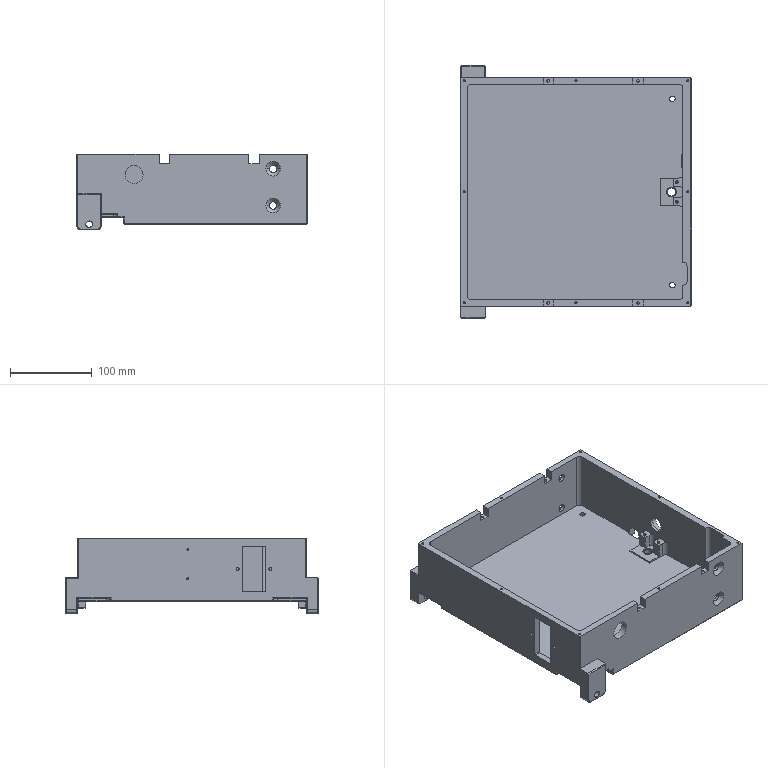NC program | Mastercam | posted with a generic post
Lines 7234 to 8037 of 104433:
(20 FEM |TOOL - 20|DIA. OFF. - 20|LEN. - 20|TOOL DIA. - 20.)
N4630 T20 M6
N4632 G0 G54 G90 X-117.9 Y-104.336 C0. B0. S4000 M3
N4634 G43 H20 Z50.
N4636 Z2.61
N4638 G1 Z2.11 F600.
N4640 X-117.911 Z1.901 F4000.
N4642 X-117.944 Z1.694
N4644 X-117.998 Z1.492
N4646 X-118.073 Z1.296
N4648 X-118.168 Z1.11
N4650 X-118.282 Z.934
N4652 X-118.414 Z.771
N4654 X-118.562 Z.623
N4656 X-118.724 Z.492
N4658 X-118.9 Z.378
N4660 X-119.087 Z.283
N4662 X-119.282 Z.208
N4664 X-119.484 Z.153
N4666 X-119.691 Z.121
N4668 X-119.9 Z.11
N4670 X-120.109 Y-104.347 Z.102
N4672 X-120.316 Y-104.38 Z.095
N4674 X-120.518 Y-104.434 Z.088
N4676 X-120.713 Y-104.509 Z.08
N4678 X-120.9 Y-104.604 Z.073
N4680 X-121.076 Y-104.718 Z.066
N4682 X-121.238 Y-104.85 Z.059
N4684 X-121.386 Y-104.998 Z.051
N4686 X-121.518 Y-105.161 Z.044
N4688 X-121.632 Y-105.336 Z.037
N4690 X-121.727 Y-105.523 Z.029
N4692 X-121.802 Y-105.718 Z.022
N4694 X-121.856 Y-105.92 Z.015
N4696 X-121.889 Y-106.127 Z.007
N4698 X-121.9 Y-106.336 Z0.
N4700 Y-120.9
N4702 G2 X-120.453 Y-120.899 I1.447 J-1517.237
N4704 X-113.75 Y-120.914 J-1517.238
N4706 X-110.741 Y-121.53 I-.477 J-9.989
N4708 G1 X-110.718 Y-121.538
N4710 G2 X-108.631 Y-122.608 I-3.486 J-9.373
N4712 G1 X-108.612 Y-122.621
N4714 G2 X-106.882 Y-124.093 I-5.573 J-8.303
N4716 G1 X-106.866 Y-124.109
N4718 G2 X-105.533 Y-125.9 I-7.304 J-6.831
N4720 G1 X-94.468
N4722 X-94.196 Y-125.462
N4724 G2 X-93.088 Y-124.06 I8.366 J-5.478
N4726 G1 X-93.072 Y-124.044
N4728 G2 X-91.448 Y-122.661 I7.258 J-6.879
N4730 G1 X-91.431 Y-122.65
N4732 G2 X-89.722 Y-121.714 I5.633 J-8.262
N4734 G1 X-89.705 Y-121.707
N4736 G2 X-87.923 Y-121.137 I3.925 J-9.198
N4738 G1 X-87.904 Y-121.133
N4740 G2 X-85.963 Y-120.903 I2.142 J-9.768
N4742 G1 X-85.271 Y-120.9
N4744 X-85.062 Y-120.888 Z.007
N4746 X-84.855 Y-120.855 Z.015
N4748 X-84.653 Y-120.8 Z.022
N4750 X-84.458 Y-120.724 Z.029
N4752 X-84.272 Y-120.628 Z.037
N4754 X-84.097 Y-120.513 Z.044
N4756 X-83.935 Y-120.381 Z.051
N4758 X-83.787 Y-120.232 Z.059
N4760 X-83.656 Y-120.069 Z.066
N4762 X-83.543 Y-119.893 Z.073
N4764 X-83.449 Y-119.706 Z.08
N4766 X-83.374 Y-119.51 Z.088
N4768 X-83.321 Y-119.308 Z.095
N4770 X-83.289 Y-119.101 Z.102
N4772 X-83.279 Y-118.892 Z.11
N4774 X-83.28 Y-118.683 Z.121
N4776 X-83.281 Y-118.476 Z.153
N4778 Y-118.274 Z.208
N4780 X-83.282 Y-118.079 Z.283
N4782 X-83.283 Y-117.892 Z.378
N4784 X-83.284 Y-117.716 Z.492
N4786 Y-117.554 Z.623
N4788 X-83.285 Y-117.406 Z.771
N4790 X-83.286 Y-117.274 Z.934
N4792 Y-117.16 Z1.11
N4794 Y-117.065 Z1.296
N4796 X-83.287 Y-116.99 Z1.492
N4798 Y-116.936 Z1.694
N4800 Y-116.903 Z1.901
N4802 Y-116.892 Z2.11
N4804 Z2.61
N4806 Z2.86
N4808 Z1.61
N4810 Z1.11 F600.
N4812 Y-116.903 Z.901 F4000.
N4814 Y-116.936 Z.694
N4816 Y-116.99 Z.492
N4818 X-83.286 Y-117.065 Z.296
N4820 Y-117.16 Z.11
N4822 Y-117.274 Z-.066
N4824 X-83.285 Y-117.406 Z-.229
N4826 X-83.284 Y-117.554 Z-.377
N4828 Y-117.716 Z-.508
N4830 X-83.283 Y-117.892 Z-.622
N4832 X-83.282 Y-118.079 Z-.717
N4834 X-83.281 Y-118.274 Z-.792
N4836 Y-118.476 Z-.847
N4838 X-83.28 Y-118.683 Z-.879
N4840 X-83.279 Y-118.892 Z-.89
N4842 X-83.289 Y-119.101 Z-.898
N4844 X-83.321 Y-119.308 Z-.905
N4846 X-83.374 Y-119.51 Z-.912
N4848 X-83.449 Y-119.706 Z-.92
N4850 X-83.543 Y-119.893 Z-.927
N4852 X-83.656 Y-120.069 Z-.934
N4854 X-83.787 Y-120.232 Z-.941
N4856 X-83.935 Y-120.381 Z-.949
N4858 X-84.097 Y-120.513 Z-.956
N4860 X-84.272 Y-120.628 Z-.963
N4862 X-84.458 Y-120.724 Z-.971
N4864 X-84.653 Y-120.8 Z-.978
N4866 X-84.855 Y-120.855 Z-.985
N4868 X-85.062 Y-120.888 Z-.993
N4870 X-85.271 Y-120.9 Z-1.
N4872 X-85.963 Y-120.903
N4874 G3 X-87.904 Y-121.133 I.201 J-9.998
N4876 G1 X-87.923 Y-121.137
N4878 G3 X-89.705 Y-121.707 I2.143 J-9.768
N4880 G1 X-89.722 Y-121.714
N4882 G3 X-91.431 Y-122.65 I3.924 J-9.198
N4884 G1 X-91.448 Y-122.661
N4886 G3 X-93.072 Y-124.044 I5.634 J-8.262
N4888 G1 X-93.088 Y-124.06
N4890 G3 X-94.196 Y-125.462 I7.258 J-6.88
N4892 G1 X-94.468 Y-125.9
N4894 X-105.533
N4896 G3 X-106.866 Y-124.109 I-8.637 J-5.04
N4898 G1 X-106.882 Y-124.093
N4900 G3 X-108.612 Y-122.621 I-7.303 J-6.831
N4902 G1 X-108.631 Y-122.608
N4904 G3 X-110.718 Y-121.538 I-5.573 J-8.303
N4906 G1 X-110.741 Y-121.53
N4908 G3 X-113.75 Y-120.914 I-3.486 J-9.373
N4910 X-120.453 Y-120.899 I-6.703 J-1517.224
N4912 X-121.9 Y-120.9 J-1517.239
N4914 G1 Y-106.336
N4916 X-121.875 Y-106.023 Z-.989
N4918 X-121.802 Y-105.718 Z-.978
N4920 X-121.682 Y-105.428 Z-.967
N4922 X-121.518 Y-105.161 Z-.956
N4924 X-121.314 Y-104.922 Z-.945
N4926 X-121.076 Y-104.718 Z-.934
N4928 X-120.808 Y-104.554 Z-.923
N4930 X-120.518 Y-104.434 Z-.912
N4932 X-120.213 Y-104.361 Z-.901
N4934 X-119.9 Y-104.336 Z-.89
N4936 X-119.691 Z-.879
N4938 X-119.484 Z-.847
N4940 X-119.282 Z-.792
N4942 X-119.087 Z-.717
N4944 X-118.9 Z-.622
N4946 X-118.724 Z-.508
N4948 X-118.562 Z-.377
N4950 X-118.414 Z-.229
N4952 X-118.282 Z-.066
N4954 X-118.168 Z.11
N4956 X-118.073 Z.296
N4958 X-117.998 Z.492
N4960 X-117.944 Z.694
N4962 X-117.911 Z.901
N4964 X-117.9 Z1.11
N4966 Z1.61
N4968 Z1.86
N4970 Z.61
N4972 Z.11 F600.
N4974 X-117.911 Z-.099 F4000.
N4976 X-117.944 Z-.306
N4978 X-117.998 Z-.508
N4980 X-118.073 Z-.704
N4982 X-118.168 Z-.89
N4984 X-118.282 Z-1.066
N4986 X-118.414 Z-1.229
N4988 X-118.562 Z-1.377
N4990 X-118.724 Z-1.508
N4992 X-118.9 Z-1.622
N4994 X-119.087 Z-1.717
N4996 X-119.282 Z-1.792
N4998 X-119.484 Z-1.847
N5000 X-119.691 Z-1.879
N5002 X-119.9 Z-1.89
N5004 X-120.109 Y-104.347 Z-1.898
N5006 X-120.316 Y-104.38 Z-1.905
N5008 X-120.518 Y-104.434 Z-1.912
N5010 X-120.713 Y-104.509 Z-1.92
N5012 X-120.9 Y-104.604 Z-1.927
N5014 X-121.076 Y-104.718 Z-1.934
N5016 X-121.238 Y-104.85 Z-1.941
N5018 X-121.386 Y-104.998 Z-1.949
N5020 X-121.518 Y-105.161 Z-1.956
N5022 X-121.632 Y-105.336 Z-1.963
N5024 X-121.727 Y-105.523 Z-1.971
N5026 X-121.802 Y-105.718 Z-1.978
N5028 X-121.856 Y-105.92 Z-1.985
N5030 X-121.889 Y-106.127 Z-1.993
N5032 X-121.9 Y-106.336 Z-2.
N5034 Y-120.9
N5036 G2 X-120.453 Y-120.899 I1.447 J-1517.238
N5038 X-113.75 Y-120.914 J-1517.239
N5040 X-110.741 Y-121.53 I-.477 J-9.989
N5042 G1 X-110.718 Y-121.538
N5044 G2 X-108.631 Y-122.608 I-3.486 J-9.373
N5046 G1 X-108.612 Y-122.621
N5048 G2 X-106.882 Y-124.093 I-5.573 J-8.303
N5050 G1 X-106.866 Y-124.109
N5052 G2 X-105.533 Y-125.9 I-7.304 J-6.831
N5054 G1 X-94.468
N5056 X-94.196 Y-125.462
N5058 G2 X-93.088 Y-124.06 I8.366 J-5.478
N5060 G1 X-93.072 Y-124.044
N5062 G2 X-91.448 Y-122.661 I7.258 J-6.879
N5064 G1 X-91.431 Y-122.65
N5066 G2 X-89.722 Y-121.714 I5.633 J-8.262
N5068 G1 X-89.705 Y-121.707
N5070 G2 X-87.923 Y-121.137 I3.925 J-9.198
N5072 G1 X-87.904 Y-121.133
N5074 G2 X-85.963 Y-120.903 I2.142 J-9.768
N5076 G1 X-85.271 Y-120.9
N5078 X-85.062 Y-120.888 Z-1.993
N5080 X-84.855 Y-120.855 Z-1.985
N5082 X-84.653 Y-120.8 Z-1.978
N5084 X-84.458 Y-120.724 Z-1.971
N5086 X-84.272 Y-120.628 Z-1.963
N5088 X-84.097 Y-120.513 Z-1.956
N5090 X-83.935 Y-120.381 Z-1.949
N5092 X-83.787 Y-120.232 Z-1.941
N5094 X-83.656 Y-120.069 Z-1.934
N5096 X-83.543 Y-119.893 Z-1.927
N5098 X-83.449 Y-119.706 Z-1.92
N5100 X-83.374 Y-119.51 Z-1.912
N5102 X-83.321 Y-119.308 Z-1.905
N5104 X-83.289 Y-119.101 Z-1.898
N5106 X-83.279 Y-118.892 Z-1.89
N5108 X-83.28 Y-118.683 Z-1.879
N5110 X-83.281 Y-118.476 Z-1.847
N5112 Y-118.274 Z-1.792
N5114 X-83.282 Y-118.079 Z-1.717
N5116 X-83.283 Y-117.892 Z-1.622
N5118 X-83.284 Y-117.716 Z-1.508
N5120 Y-117.554 Z-1.377
N5122 X-83.285 Y-117.406 Z-1.229
N5124 X-83.286 Y-117.274 Z-1.066
N5126 Y-117.16 Z-.89
N5128 Y-117.065 Z-.704
N5130 X-83.287 Y-116.99 Z-.508
N5132 Y-116.936 Z-.306
N5134 Y-116.903 Z-.099
N5136 Y-116.892 Z.11
N5138 Z.61
N5140 Z.86
N5142 Z-.39
N5144 Z-.89 F600.
N5146 Y-116.903 Z-1.099 F4000.
N5148 Y-116.936 Z-1.306
N5150 Y-116.99 Z-1.508
N5152 X-83.286 Y-117.065 Z-1.704
N5154 Y-117.16 Z-1.89
N5156 Y-117.274 Z-2.066
N5158 X-83.285 Y-117.406 Z-2.229
N5160 X-83.284 Y-117.554 Z-2.377
N5162 Y-117.716 Z-2.508
N5164 X-83.283 Y-117.892 Z-2.622
N5166 X-83.282 Y-118.079 Z-2.717
N5168 X-83.281 Y-118.274 Z-2.792
N5170 Y-118.476 Z-2.847
N5172 X-83.28 Y-118.683 Z-2.879
N5174 X-83.279 Y-118.892 Z-2.89
N5176 X-83.289 Y-119.101 Z-2.898
N5178 X-83.321 Y-119.308 Z-2.905
N5180 X-83.374 Y-119.51 Z-2.912
N5182 X-83.449 Y-119.706 Z-2.92
N5184 X-83.543 Y-119.893 Z-2.927
N5186 X-83.656 Y-120.069 Z-2.934
N5188 X-83.787 Y-120.232 Z-2.941
N5190 X-83.935 Y-120.381 Z-2.949
N5192 X-84.097 Y-120.513 Z-2.956
N5194 X-84.272 Y-120.628 Z-2.963
N5196 X-84.458 Y-120.724 Z-2.971
N5198 X-84.653 Y-120.8 Z-2.978
N5200 X-84.855 Y-120.855 Z-2.985
N5202 X-85.062 Y-120.888 Z-2.993
N5204 X-85.271 Y-120.9 Z-3.
N5206 X-85.963 Y-120.903
N5208 G3 X-87.904 Y-121.133 I.201 J-9.998
N5210 G1 X-87.923 Y-121.137
N5212 G3 X-89.705 Y-121.707 I2.143 J-9.768
N5214 G1 X-89.722 Y-121.714
N5216 G3 X-91.431 Y-122.65 I3.924 J-9.198
N5218 G1 X-91.448 Y-122.661
N5220 G3 X-93.072 Y-124.044 I5.634 J-8.262
N5222 G1 X-93.088 Y-124.06
N5224 G3 X-94.196 Y-125.462 I7.258 J-6.88
N5226 G1 X-94.468 Y-125.9
N5228 X-105.533
N5230 G3 X-106.866 Y-124.109 I-8.637 J-5.04
N5232 G1 X-106.882 Y-124.093
N5234 G3 X-108.612 Y-122.621 I-7.303 J-6.831
N5236 G1 X-108.631 Y-122.608
N5238 G3 X-110.718 Y-121.538 I-5.573 J-8.303
N5240 G1 X-110.741 Y-121.53
N5242 G3 X-113.75 Y-120.914 I-3.486 J-9.373
N5244 X-120.453 Y-120.899 I-6.703 J-1517.224
N5246 X-121.9 Y-120.9 J-1517.239
N5248 G1 Y-106.336
N5250 X-121.875 Y-106.023 Z-2.989
N5252 X-121.802 Y-105.718 Z-2.978
N5254 X-121.682 Y-105.428 Z-2.967
N5256 X-121.518 Y-105.161 Z-2.956
N5258 X-121.314 Y-104.922 Z-2.945
N5260 X-121.076 Y-104.718 Z-2.934
N5262 X-120.808 Y-104.554 Z-2.923
N5264 X-120.518 Y-104.434 Z-2.912
N5266 X-120.213 Y-104.361 Z-2.901
N5268 X-119.9 Y-104.336 Z-2.89
N5270 X-119.691 Z-2.879
N5272 X-119.484 Z-2.847
N5274 X-119.282 Z-2.792
N5276 X-119.087 Z-2.717
N5278 X-118.9 Z-2.622
N5280 X-118.724 Z-2.508
N5282 X-118.562 Z-2.377
N5284 X-118.414 Z-2.229
N5286 X-118.282 Z-2.066
N5288 X-118.168 Z-1.89
N5290 X-118.073 Z-1.704
N5292 X-117.998 Z-1.508
N5294 X-117.944 Z-1.306
N5296 X-117.911 Z-1.099
N5298 X-117.9 Z-.89
N5300 Z-.39
N5302 Z-.14
N5304 Z-1.39
N5306 Z-1.89 F600.
N5308 X-117.911 Z-2.099 F4000.
N5310 X-117.944 Z-2.306
N5312 X-117.998 Z-2.508
N5314 X-118.073 Z-2.704
N5316 X-118.168 Z-2.89
N5318 X-118.282 Z-3.066
N5320 X-118.414 Z-3.229
N5322 X-118.562 Z-3.377
N5324 X-118.724 Z-3.508
N5326 X-118.9 Z-3.622
N5328 X-119.087 Z-3.717
N5330 X-119.282 Z-3.792
N5332 X-119.484 Z-3.847
N5334 X-119.691 Z-3.879
N5336 X-119.9 Z-3.89
N5338 X-120.109 Y-104.347 Z-3.898
N5340 X-120.316 Y-104.38 Z-3.905
N5342 X-120.518 Y-104.434 Z-3.912
N5344 X-120.713 Y-104.509 Z-3.92
N5346 X-120.9 Y-104.604 Z-3.927
N5348 X-121.076 Y-104.718 Z-3.934
N5350 X-121.238 Y-104.85 Z-3.941
N5352 X-121.386 Y-104.998 Z-3.949
N5354 X-121.518 Y-105.161 Z-3.956
N5356 X-121.632 Y-105.336 Z-3.963
N5358 X-121.727 Y-105.523 Z-3.971
N5360 X-121.802 Y-105.718 Z-3.978
N5362 X-121.856 Y-105.92 Z-3.985
N5364 X-121.889 Y-106.127 Z-3.993
N5366 X-121.9 Y-106.336 Z-4.
N5368 Y-120.9
N5370 G2 X-120.453 Y-120.899 I1.447 J-1517.238
N5372 X-113.75 Y-120.914 J-1517.239
N5374 X-110.741 Y-121.53 I-.477 J-9.989
N5376 G1 X-110.718 Y-121.538
N5378 G2 X-108.631 Y-122.608 I-3.486 J-9.373
N5380 G1 X-108.612 Y-122.621
N5382 G2 X-106.882 Y-124.093 I-5.573 J-8.303
N5384 G1 X-106.866 Y-124.109
N5386 G2 X-105.533 Y-125.9 I-7.304 J-6.831
N5388 G1 X-94.468
N5390 X-94.196 Y-125.462
N5392 G2 X-93.088 Y-124.06 I8.366 J-5.478
N5394 G1 X-93.072 Y-124.044
N5396 G2 X-91.448 Y-122.661 I7.258 J-6.879
N5398 G1 X-91.431 Y-122.65
N5400 G2 X-89.722 Y-121.714 I5.633 J-8.262
N5402 G1 X-89.705 Y-121.707
N5404 G2 X-87.923 Y-121.137 I3.925 J-9.198
N5406 G1 X-87.904 Y-121.133
N5408 G2 X-85.963 Y-120.903 I2.142 J-9.768
N5410 G1 X-85.271 Y-120.9
N5412 X-85.062 Y-120.888 Z-3.993
N5414 X-84.855 Y-120.855 Z-3.985
N5416 X-84.653 Y-120.8 Z-3.978
N5418 X-84.458 Y-120.724 Z-3.971
N5420 X-84.272 Y-120.628 Z-3.963
N5422 X-84.097 Y-120.513 Z-3.956
N5424 X-83.935 Y-120.381 Z-3.949
N5426 X-83.787 Y-120.232 Z-3.941
N5428 X-83.656 Y-120.069 Z-3.934
N5430 X-83.543 Y-119.893 Z-3.927
N5432 X-83.449 Y-119.706 Z-3.92
N5434 X-83.374 Y-119.51 Z-3.912
N5436 X-83.321 Y-119.308 Z-3.905
N5438 X-83.289 Y-119.101 Z-3.898
N5440 X-83.279 Y-118.892 Z-3.89
N5442 X-83.28 Y-118.683 Z-3.879
N5444 X-83.281 Y-118.476 Z-3.847
N5446 Y-118.274 Z-3.792
N5448 X-83.282 Y-118.079 Z-3.717
N5450 X-83.283 Y-117.892 Z-3.622
N5452 X-83.284 Y-117.716 Z-3.508
N5454 Y-117.554 Z-3.377
N5456 X-83.285 Y-117.406 Z-3.229
N5458 X-83.286 Y-117.274 Z-3.066
N5460 Y-117.16 Z-2.89
N5462 Y-117.065 Z-2.704
N5464 X-83.287 Y-116.99 Z-2.508
N5466 Y-116.936 Z-2.306
N5468 Y-116.903 Z-2.099
N5470 Y-116.892 Z-1.89
N5472 Z-1.39
N5474 Z-1.14
N5476 Z-2.39
N5478 Z-2.89 F600.
N5480 Y-116.903 Z-3.099 F4000.
N5482 Y-116.936 Z-3.306
N5484 Y-116.99 Z-3.508
N5486 X-83.286 Y-117.065 Z-3.704
N5488 Y-117.16 Z-3.89
N5490 Y-117.274 Z-4.066
N5492 X-83.285 Y-117.406 Z-4.229
N5494 X-83.284 Y-117.554 Z-4.377
N5496 Y-117.716 Z-4.508
N5498 X-83.283 Y-117.892 Z-4.622
N5500 X-83.282 Y-118.079 Z-4.717
N5502 X-83.281 Y-118.274 Z-4.792
N5504 Y-118.476 Z-4.847
N5506 X-83.28 Y-118.683 Z-4.879
N5508 X-83.279 Y-118.892 Z-4.89
N5510 X-83.289 Y-119.101 Z-4.898
N5512 X-83.321 Y-119.308 Z-4.905
N5514 X-83.374 Y-119.51 Z-4.912
N5516 X-83.449 Y-119.706 Z-4.92
N5518 X-83.543 Y-119.893 Z-4.927
N5520 X-83.656 Y-120.069 Z-4.934
N5522 X-83.787 Y-120.232 Z-4.941
N5524 X-83.935 Y-120.381 Z-4.949
N5526 X-84.097 Y-120.513 Z-4.956
N5528 X-84.272 Y-120.628 Z-4.963
N5530 X-84.458 Y-120.724 Z-4.971
N5532 X-84.653 Y-120.8 Z-4.978
N5534 X-84.855 Y-120.855 Z-4.985
N5536 X-85.062 Y-120.888 Z-4.993
N5538 X-85.271 Y-120.9 Z-5.
N5540 X-85.963 Y-120.903
N5542 G3 X-87.904 Y-121.133 I.201 J-9.998
N5544 G1 X-87.923 Y-121.137
N5546 G3 X-89.705 Y-121.707 I2.143 J-9.768
N5548 G1 X-89.722 Y-121.714
N5550 G3 X-91.431 Y-122.65 I3.924 J-9.198
N5552 G1 X-91.448 Y-122.661
N5554 G3 X-93.072 Y-124.044 I5.634 J-8.262
N5556 G1 X-93.088 Y-124.06
N5558 G3 X-94.196 Y-125.462 I7.258 J-6.88
N5560 G1 X-94.468 Y-125.9
N5562 X-105.533
N5564 G3 X-106.866 Y-124.109 I-8.637 J-5.04
N5566 G1 X-106.882 Y-124.093
N5568 G3 X-108.612 Y-122.621 I-7.303 J-6.831
N5570 G1 X-108.631 Y-122.608
N5572 G3 X-110.718 Y-121.538 I-5.573 J-8.303
N5574 G1 X-110.741 Y-121.53
N5576 G3 X-113.75 Y-120.914 I-3.486 J-9.373
N5578 X-120.453 Y-120.899 I-6.703 J-1517.224
N5580 X-121.9 Y-120.9 J-1517.239
N5582 G1 Y-106.336
N5584 X-121.875 Y-106.023 Z-4.989
N5586 X-121.802 Y-105.718 Z-4.978
N5588 X-121.682 Y-105.428 Z-4.967
N5590 X-121.518 Y-105.161 Z-4.956
N5592 X-121.314 Y-104.922 Z-4.945
N5594 X-121.076 Y-104.718 Z-4.934
N5596 X-120.808 Y-104.554 Z-4.923
N5598 X-120.518 Y-104.434 Z-4.912
N5600 X-120.213 Y-104.361 Z-4.901
N5602 X-119.9 Y-104.336 Z-4.89
N5604 X-119.691 Z-4.879
N5606 X-119.484 Z-4.847
N5608 X-119.282 Z-4.792
N5610 X-119.087 Z-4.717
N5612 X-118.9 Z-4.622
N5614 X-118.724 Z-4.508
N5616 X-118.562 Z-4.377
N5618 X-118.414 Z-4.229
N5620 X-118.282 Z-4.066
N5622 X-118.168 Z-3.89
N5624 X-118.073 Z-3.704
N5626 X-117.998 Z-3.508
N5628 X-117.944 Z-3.306
N5630 X-117.911 Z-3.099
N5632 X-117.9 Z-2.89
N5634 Z-2.39
N5636 Z-2.14
N5638 Z-3.39
N5640 Z-3.89 F600.
N5642 X-117.911 Z-4.099 F4000.
N5644 X-117.944 Z-4.306
N5646 X-117.998 Z-4.508
N5648 X-118.073 Z-4.704
N5650 X-118.168 Z-4.89
N5652 X-118.282 Z-5.066
N5654 X-118.414 Z-5.229
N5656 X-118.562 Z-5.377
N5658 X-118.724 Z-5.508
N5660 X-118.9 Z-5.622
N5662 X-119.087 Z-5.717
N5664 X-119.282 Z-5.792
N5666 X-119.484 Z-5.847
N5668 X-119.691 Z-5.879
N5670 X-119.9 Z-5.89
N5672 X-120.109 Y-104.347 Z-5.898
N5674 X-120.316 Y-104.38 Z-5.905
N5676 X-120.518 Y-104.434 Z-5.912
N5678 X-120.713 Y-104.509 Z-5.92
N5680 X-120.9 Y-104.604 Z-5.927
N5682 X-121.076 Y-104.718 Z-5.934
N5684 X-121.238 Y-104.85 Z-5.941
N5686 X-121.386 Y-104.998 Z-5.949
N5688 X-121.518 Y-105.161 Z-5.956
N5690 X-121.632 Y-105.336 Z-5.963
N5692 X-121.727 Y-105.523 Z-5.971
N5694 X-121.802 Y-105.718 Z-5.978
N5696 X-121.856 Y-105.92 Z-5.985
N5698 X-121.889 Y-106.127 Z-5.993
N5700 X-121.9 Y-106.336 Z-6.
N5702 Y-120.9
N5704 G2 X-120.453 Y-120.899 I1.447 J-1517.238
N5706 X-113.75 Y-120.914 J-1517.239
N5708 X-110.741 Y-121.53 I-.477 J-9.989
N5710 G1 X-110.718 Y-121.538
N5712 G2 X-108.631 Y-122.608 I-3.486 J-9.373
N5714 G1 X-108.612 Y-122.621
N5716 G2 X-106.882 Y-124.093 I-5.573 J-8.303
N5718 G1 X-106.866 Y-124.109
N5720 G2 X-105.533 Y-125.9 I-7.304 J-6.831
N5722 G1 X-94.468
N5724 X-94.196 Y-125.462
N5726 G2 X-93.088 Y-124.06 I8.366 J-5.478
N5728 G1 X-93.072 Y-124.044
N5730 G2 X-91.448 Y-122.661 I7.258 J-6.879
N5732 G1 X-91.431 Y-122.65
N5734 G2 X-89.722 Y-121.714 I5.633 J-8.262
N5736 G1 X-89.705 Y-121.707
N5738 G2 X-87.923 Y-121.137 I3.925 J-9.198
N5740 G1 X-87.904 Y-121.133
N5742 G2 X-85.963 Y-120.903 I2.142 J-9.768
N5744 G1 X-85.271 Y-120.9
N5746 X-85.062 Y-120.888 Z-5.993
N5748 X-84.855 Y-120.855 Z-5.985
N5750 X-84.653 Y-120.8 Z-5.978
N5752 X-84.458 Y-120.724 Z-5.971
N5754 X-84.272 Y-120.628 Z-5.963
N5756 X-84.097 Y-120.513 Z-5.956
N5758 X-83.935 Y-120.381 Z-5.949
N5760 X-83.787 Y-120.232 Z-5.941
N5762 X-83.656 Y-120.069 Z-5.934
N5764 X-83.543 Y-119.893 Z-5.927
N5766 X-83.449 Y-119.706 Z-5.92
N5768 X-83.374 Y-119.51 Z-5.912
N5770 X-83.321 Y-119.308 Z-5.905
N5772 X-83.289 Y-119.101 Z-5.898
N5774 X-83.279 Y-118.892 Z-5.89
N5776 X-83.28 Y-118.683 Z-5.879
N5778 X-83.281 Y-118.476 Z-5.847
N5780 Y-118.274 Z-5.792
N5782 X-83.282 Y-118.079 Z-5.717
N5784 X-83.283 Y-117.892 Z-5.622
N5786 X-83.284 Y-117.716 Z-5.508
N5788 Y-117.554 Z-5.377
N5790 X-83.285 Y-117.406 Z-5.229
N5792 X-83.286 Y-117.274 Z-5.066
N5794 Y-117.16 Z-4.89
N5796 Y-117.065 Z-4.704
N5798 X-83.287 Y-116.99 Z-4.508
N5800 Y-116.936 Z-4.306
N5802 Y-116.903 Z-4.099
N5804 Y-116.892 Z-3.89
N5806 Z-3.39
N5808 Z-3.14
N5810 Z-4.39
N5812 Z-4.89 F600.
N5814 Y-116.903 Z-5.099 F4000.
N5816 Y-116.936 Z-5.306
N5818 Y-116.99 Z-5.508
N5820 X-83.286 Y-117.065 Z-5.704
N5822 Y-117.16 Z-5.89
N5824 Y-117.274 Z-6.066
N5826 X-83.285 Y-117.406 Z-6.229
N5828 X-83.284 Y-117.554 Z-6.377
N5830 Y-117.716 Z-6.508
N5832 X-83.283 Y-117.892 Z-6.622
N5834 X-83.282 Y-118.079 Z-6.717
N5836 X-83.281 Y-118.274 Z-6.792
N5838 Y-118.476 Z-6.847
N5840 X-83.28 Y-118.683 Z-6.879
N5842 X-83.279 Y-118.892 Z-6.89
N5844 X-83.289 Y-119.101 Z-6.898
N5846 X-83.321 Y-119.308 Z-6.905
N5848 X-83.374 Y-119.51 Z-6.912
N5850 X-83.449 Y-119.706 Z-6.92
N5852 X-83.543 Y-119.893 Z-6.927
N5854 X-83.656 Y-120.069 Z-6.934
N5856 X-83.787 Y-120.232 Z-6.941
N5858 X-83.935 Y-120.381 Z-6.949
N5860 X-84.097 Y-120.513 Z-6.956
N5862 X-84.272 Y-120.628 Z-6.963
N5864 X-84.458 Y-120.724 Z-6.971
N5866 X-84.653 Y-120.8 Z-6.978
N5868 X-84.855 Y-120.855 Z-6.985
N5870 X-85.062 Y-120.888 Z-6.993
N5872 X-85.271 Y-120.9 Z-7.
N5874 X-85.963 Y-120.903
N5876 G3 X-87.904 Y-121.133 I.201 J-9.998
N5878 G1 X-87.923 Y-121.137
N5880 G3 X-89.705 Y-121.707 I2.143 J-9.768
N5882 G1 X-89.722 Y-121.714
N5884 G3 X-91.431 Y-122.65 I3.924 J-9.198
N5886 G1 X-91.448 Y-122.661
N5888 G3 X-93.072 Y-124.044 I5.634 J-8.262
N5890 G1 X-93.088 Y-124.06
N5892 G3 X-94.196 Y-125.462 I7.258 J-6.88
N5894 G1 X-94.468 Y-125.9
N5896 X-105.533
N5898 G3 X-106.866 Y-124.109 I-8.637 J-5.04
N5900 G1 X-106.882 Y-124.093
N5902 G3 X-108.612 Y-122.621 I-7.303 J-6.831
N5904 G1 X-108.631 Y-122.608
N5906 G3 X-110.718 Y-121.538 I-5.573 J-8.303
N5908 G1 X-110.741 Y-121.53
N5910 G3 X-113.75 Y-120.914 I-3.486 J-9.373
N5912 X-120.453 Y-120.899 I-6.703 J-1517.224
N5914 X-121.9 Y-120.9 J-1517.239
N5916 G1 Y-106.336
N5918 X-121.875 Y-106.023 Z-6.989
N5920 X-121.802 Y-105.718 Z-6.978
N5922 X-121.682 Y-105.428 Z-6.967
N5924 X-121.518 Y-105.161 Z-6.956
N5926 X-121.314 Y-104.922 Z-6.945
N5928 X-121.076 Y-104.718 Z-6.934
N5930 X-120.808 Y-104.554 Z-6.923
N5932 X-120.518 Y-104.434 Z-6.912
N5934 X-120.213 Y-104.361 Z-6.901
N5936 X-119.9 Y-104.336 Z-6.89
N5938 X-119.691 Z-6.879
N5940 X-119.484 Z-6.847
N5942 X-119.282 Z-6.792
N5944 X-119.087 Z-6.717
N5946 X-118.9 Z-6.622
N5948 X-118.724 Z-6.508
N5950 X-118.562 Z-6.377
N5952 X-118.414 Z-6.229
N5954 X-118.282 Z-6.066
N5956 X-118.168 Z-5.89
N5958 X-118.073 Z-5.704
N5960 X-117.998 Z-5.508
N5962 X-117.944 Z-5.306
N5964 X-117.911 Z-5.099
N5966 X-117.9 Z-4.89
N5968 Z-4.39
N5970 Z-4.14
N5972 Z-5.39
N5974 Z-5.89 F600.
N5976 X-117.911 Z-6.099 F4000.
N5978 X-117.944 Z-6.306
N5980 X-117.998 Z-6.508
N5982 X-118.073 Z-6.704
N5984 X-118.168 Z-6.89
N5986 X-118.282 Z-7.066
N5988 X-118.414 Z-7.229
N5990 X-118.562 Z-7.377
N5992 X-118.724 Z-7.508
N5994 X-118.9 Z-7.622
N5996 X-119.087 Z-7.717
N5998 X-119.282 Z-7.792
N6000 X-119.484 Z-7.847
N6002 X-119.691 Z-7.879
N6004 X-119.9 Z-7.89
N6006 X-120.109 Y-104.347 Z-7.898
N6008 X-120.316 Y-104.38 Z-7.905
N6010 X-120.518 Y-104.434 Z-7.912
N6012 X-120.713 Y-104.509 Z-7.92
N6014 X-120.9 Y-104.604 Z-7.927
N6016 X-121.076 Y-104.718 Z-7.934
N6018 X-121.238 Y-104.85 Z-7.941
N6020 X-121.386 Y-104.998 Z-7.949
N6022 X-121.518 Y-105.161 Z-7.956
N6024 X-121.632 Y-105.336 Z-7.963
N6026 X-121.727 Y-105.523 Z-7.971
N6028 X-121.802 Y-105.718 Z-7.978
N6030 X-121.856 Y-105.92 Z-7.985
N6032 X-121.889 Y-106.127 Z-7.993
N6034 X-121.9 Y-106.336 Z-8.
N6036 Y-120.9
N6038 G2 X-120.453 Y-120.899 I1.447 J-1517.238
N6040 X-113.75 Y-120.914 J-1517.239
N6042 X-110.741 Y-121.53 I-.477 J-9.989
N6044 G1 X-110.718 Y-121.538
N6046 G2 X-108.631 Y-122.608 I-3.486 J-9.373
N6048 G1 X-108.612 Y-122.621
N6050 G2 X-106.882 Y-124.093 I-5.573 J-8.303
N6052 G1 X-106.866 Y-124.109
N6054 G2 X-105.533 Y-125.9 I-7.304 J-6.831
N6056 G1 X-94.468
N6058 X-94.196 Y-125.462
N6060 G2 X-93.088 Y-124.06 I8.366 J-5.478
N6062 G1 X-93.072 Y-124.044
N6064 G2 X-91.448 Y-122.661 I7.258 J-6.879
N6066 G1 X-91.431 Y-122.65
N6068 G2 X-89.722 Y-121.714 I5.633 J-8.262
N6070 G1 X-89.705 Y-121.707
N6072 G2 X-87.923 Y-121.137 I3.925 J-9.198
N6074 G1 X-87.904 Y-121.133
N6076 G2 X-85.963 Y-120.903 I2.142 J-9.768
N6078 G1 X-85.271 Y-120.9
N6080 X-85.062 Y-120.888 Z-7.993
N6082 X-84.855 Y-120.855 Z-7.985
N6084 X-84.653 Y-120.8 Z-7.978
N6086 X-84.458 Y-120.724 Z-7.971
N6088 X-84.272 Y-120.628 Z-7.963
N6090 X-84.097 Y-120.513 Z-7.956
N6092 X-83.935 Y-120.381 Z-7.949
N6094 X-83.787 Y-120.232 Z-7.941
N6096 X-83.656 Y-120.069 Z-7.934
N6098 X-83.543 Y-119.893 Z-7.927
N6100 X-83.449 Y-119.706 Z-7.92
N6102 X-83.374 Y-119.51 Z-7.912
N6104 X-83.321 Y-119.308 Z-7.905
N6106 X-83.289 Y-119.101 Z-7.898
N6108 X-83.279 Y-118.892 Z-7.89
N6110 X-83.28 Y-118.683 Z-7.879
N6112 X-83.281 Y-118.476 Z-7.847
N6114 Y-118.274 Z-7.792
N6116 X-83.282 Y-118.079 Z-7.717
N6118 X-83.283 Y-117.892 Z-7.622
N6120 X-83.284 Y-117.716 Z-7.508
N6122 Y-117.554 Z-7.377
N6124 X-83.285 Y-117.406 Z-7.229
N6126 X-83.286 Y-117.274 Z-7.066
N6128 Y-117.16 Z-6.89
N6130 Y-117.065 Z-6.704
N6132 X-83.287 Y-116.99 Z-6.508
N6134 Y-116.936 Z-6.306
N6136 Y-116.903 Z-6.099
N6138 Y-116.892 Z-5.89
N6140 Z-5.39
N6142 Z-5.14
N6144 Z-6.39
N6146 Z-6.89 F600.
N6148 Y-116.903 Z-7.099 F4000.
N6150 Y-116.936 Z-7.306
N6152 Y-116.99 Z-7.508
N6154 X-83.286 Y-117.065 Z-7.704
N6156 Y-117.16 Z-7.89
N6158 Y-117.274 Z-8.066
N6160 X-83.285 Y-117.406 Z-8.229
N6162 X-83.284 Y-117.554 Z-8.377
N6164 Y-117.716 Z-8.508
N6166 X-83.283 Y-117.892 Z-8.622
N6168 X-83.282 Y-118.079 Z-8.717
N6170 X-83.281 Y-118.274 Z-8.792
N6172 Y-118.476 Z-8.847
N6174 X-83.28 Y-118.683 Z-8.879
N6176 X-83.279 Y-118.892 Z-8.89
N6178 X-83.289 Y-119.101 Z-8.898
N6180 X-83.321 Y-119.308 Z-8.905
N6182 X-83.374 Y-119.51 Z-8.912
N6184 X-83.449 Y-119.706 Z-8.92
N6186 X-83.543 Y-119.893 Z-8.927
N6188 X-83.656 Y-120.069 Z-8.934
N6190 X-83.787 Y-120.232 Z-8.941
N6192 X-83.935 Y-120.381 Z-8.949
N6194 X-84.097 Y-120.513 Z-8.956
N6196 X-84.272 Y-120.628 Z-8.963
N6198 X-84.458 Y-120.724 Z-8.971
N6200 X-84.653 Y-120.8 Z-8.978
N6202 X-84.855 Y-120.855 Z-8.985
N6204 X-85.062 Y-120.888 Z-8.993
N6206 X-85.271 Y-120.9 Z-9.
N6208 X-85.963 Y-120.903
N6210 G3 X-87.904 Y-121.133 I.201 J-9.998
N6212 G1 X-87.923 Y-121.137
N6214 G3 X-89.705 Y-121.707 I2.143 J-9.768
N6216 G1 X-89.722 Y-121.714
N6218 G3 X-91.431 Y-122.65 I3.924 J-9.198
N6220 G1 X-91.448 Y-122.661
N6222 G3 X-93.072 Y-124.044 I5.634 J-8.262
N6224 G1 X-93.088 Y-124.06
N6226 G3 X-94.196 Y-125.462 I7.258 J-6.88
N6228 G1 X-94.468 Y-125.9
N6230 X-105.533
N6232 G3 X-106.866 Y-124.109 I-8.637 J-5.04
N6234 G1 X-106.882 Y-124.093